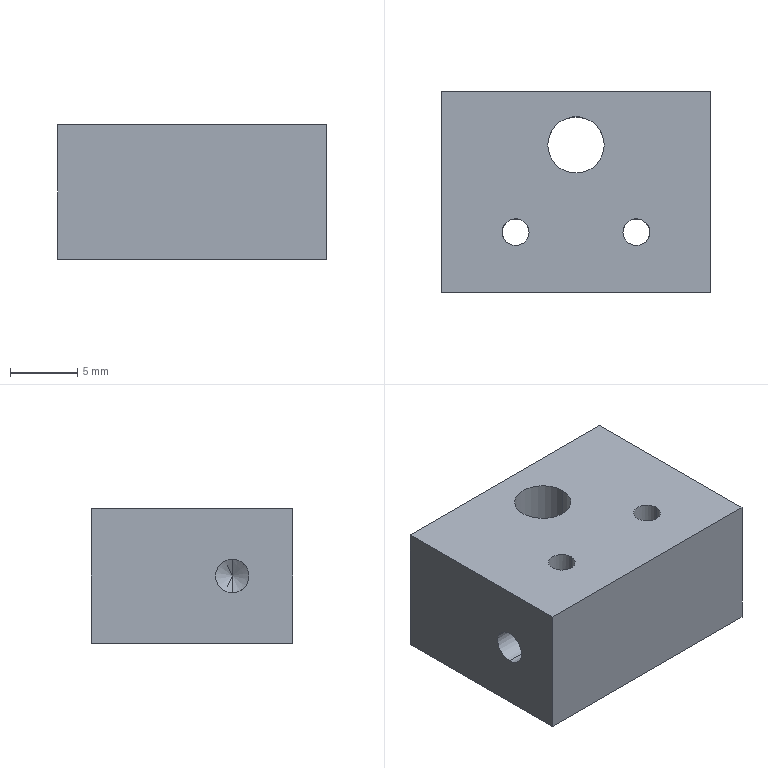Part | STEP file | D06 | 1 solid | 24 faces | box 20 x 15 x 10 mm | volume 2737 mm3 | cylinder 14 | plane 6 | cone 4 | commonest cylinder face diameters 2 x8 2.5 x4 4.2 x2